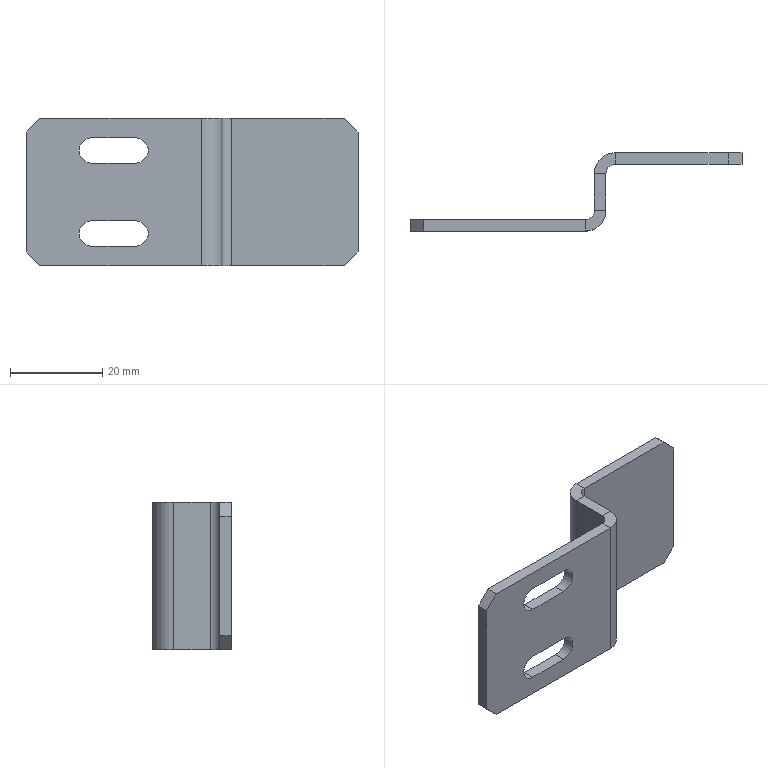Part | SolidWorks | features Chamfer 1, FlatPattern 1, HoleWzd 1, SMBaseFlange 1, SheetMetal 1 | 1 solid | 34 faces | box 72 x 17 x 32 mm | volume 6272 mm3 | plane 26 | cylinder 8 | commonest cylinder face diameters 5.5 x4 4 x2 9 x2
STEP:
#1=CARTESIAN_POINT('',(40.,2.,32.));
#2=VERTEX_POINT('',#1);
#3=CARTESIAN_POINT('',(42.5,2.,32.));
#4=VERTEX_POINT('',#3);
#5=CARTESIAN_POINT('',(40.,2.,32.));
#6=DIRECTION('',(1.,0.,0.));
#7=VECTOR('',#6,1000.);
#8=LINE('',#5,#7);
#9=EDGE_CURVE('',#2,#4,#8,.T.);
#10=ORIENTED_EDGE('',*,*,#9,.F.);
#11=CARTESIAN_POINT('',(38.,0.,32.));
#12=VERTEX_POINT('',#11);
#13=CARTESIAN_POINT('',(38.,2.,32.));
#14=DIRECTION('',(0.,0.,1.));
#15=DIRECTION('',(-1.,0.,0.));
#16=AXIS2_PLACEMENT_3D('',#13,#14,#15);
#17=CIRCLE('',#16,2.);
#18=EDGE_CURVE('',#12,#2,#17,.T.);
#19=ORIENTED_EDGE('',*,*,#18,.F.);
#20=CARTESIAN_POINT('',(38.,-2.5,32.));
#21=VERTEX_POINT('',#20);
#22=CARTESIAN_POINT('',(38.,-2.5,32.));
#23=DIRECTION('',(0.,1.,0.));
#24=VECTOR('',#23,1000.);
#25=LINE('',#22,#24);
#26=EDGE_CURVE('',#21,#12,#25,.T.);
#27=ORIENTED_EDGE('',*,*,#26,.F.);
#28=CARTESIAN_POINT('',(38.,2.,32.));
#29=DIRECTION('',(0.,0.,1.));
#30=DIRECTION('',(1.,0.,0.));
#31=AXIS2_PLACEMENT_3D('',#28,#29,#30);
#32=CIRCLE('',#31,4.5);
#33=EDGE_CURVE('',#21,#4,#32,.T.);
#34=ORIENTED_EDGE('',*,*,#33,.T.);
#35=EDGE_LOOP('',(#10,#19,#27,#34));
#36=FACE_OUTER_BOUND('',#35,.T.);
#37=CARTESIAN_POINT('',(40.,2.,32.));
#38=DIRECTION('',(0.,0.,1.));
#39=DIRECTION('',(1.,0.,0.));
#40=AXIS2_PLACEMENT_3D('',#37,#38,#39);
#41=PLANE('',#40);
#42=ADVANCED_FACE('',(#36),#41,.T.);
#43=CARTESIAN_POINT('',(40.,10.,32.));
#44=VERTEX_POINT('',#43);
#45=CARTESIAN_POINT('',(40.,0.,32.));
#46=DIRECTION('',(0.,1.,0.));
#47=VECTOR('',#46,1000.);
#48=LINE('',#45,#47);
#49=EDGE_CURVE('',#2,#44,#48,.T.);
#50=ORIENTED_EDGE('',*,*,#49,.F.);
#51=ORIENTED_EDGE('',*,*,#9,.T.);
#52=CARTESIAN_POINT('',(42.5,10.,32.));
#53=VERTEX_POINT('',#52);
#54=CARTESIAN_POINT('',(42.5,0.,32.));
#55=DIRECTION('',(0.,1.,0.));
#56=VECTOR('',#55,1000.);
#57=LINE('',#54,#56);
#58=EDGE_CURVE('',#4,#53,#57,.T.);
#59=ORIENTED_EDGE('',*,*,#58,.T.);
#60=CARTESIAN_POINT('',(42.5,10.,32.));
#61=DIRECTION('',(-1.,0.,0.));
#62=VECTOR('',#61,1000.);
#63=LINE('',#60,#62);
#64=EDGE_CURVE('',#53,#44,#63,.T.);
#65=ORIENTED_EDGE('',*,*,#64,.T.);
#66=EDGE_LOOP('',(#50,#51,#59,#65));
#67=FACE_OUTER_BOUND('',#66,.T.);
#68=CARTESIAN_POINT('',(38.,-2.5,32.));
#69=DIRECTION('',(0.,0.,1.));
#70=DIRECTION('',(1.,0.,0.));
#71=AXIS2_PLACEMENT_3D('',#68,#69,#70);
#72=PLANE('',#71);
#73=ADVANCED_FACE('',(#67),#72,.T.);
#74=CARTESIAN_POINT('',(38.,0.,0.));
#75=VERTEX_POINT('',#74);
#76=CARTESIAN_POINT('',(38.,-2.5,0.));
#77=VERTEX_POINT('',#76);
#78=CARTESIAN_POINT('',(38.,0.,0.));
#79=DIRECTION('',(0.,-1.,0.));
#80=VECTOR('',#79,1000.);
#81=LINE('',#78,#80);
#82=EDGE_CURVE('',#75,#77,#81,.T.);
#83=ORIENTED_EDGE('',*,*,#82,.F.);
#84=CARTESIAN_POINT('',(40.,2.,0.));
#85=VERTEX_POINT('',#84);
#86=CARTESIAN_POINT('',(38.,2.,0.));
#87=DIRECTION('',(0.,0.,1.));
#88=DIRECTION('',(-1.,0.,0.));
#89=AXIS2_PLACEMENT_3D('',#86,#87,#88);
#90=CIRCLE('',#89,2.);
#91=EDGE_CURVE('',#75,#85,#90,.T.);
#92=ORIENTED_EDGE('',*,*,#91,.T.);
#93=CARTESIAN_POINT('',(42.5,2.,0.));
#94=VERTEX_POINT('',#93);
#95=CARTESIAN_POINT('',(42.5,2.,0.));
#96=DIRECTION('',(-1.,0.,0.));
#97=VECTOR('',#96,1000.);
#98=LINE('',#95,#97);
#99=EDGE_CURVE('',#94,#85,#98,.T.);
#100=ORIENTED_EDGE('',*,*,#99,.F.);
#101=CARTESIAN_POINT('',(38.,2.,0.));
#102=DIRECTION('',(0.,0.,1.));
#103=DIRECTION('',(1.,0.,0.));
#104=AXIS2_PLACEMENT_3D('',#101,#102,#103);
#105=CIRCLE('',#104,4.5);
#106=EDGE_CURVE('',#77,#94,#105,.T.);
#107=ORIENTED_EDGE('',*,*,#106,.F.);
#108=EDGE_LOOP('',(#83,#92,#100,#107));
#109=FACE_OUTER_BOUND('',#108,.T.);
#110=CARTESIAN_POINT('',(38.,0.,0.));
#111=DIRECTION('',(0.,0.,-1.));
#112=DIRECTION('',(-1.,0.,0.));
#113=AXIS2_PLACEMENT_3D('',#110,#111,#112);
#114=PLANE('',#113);
#115=ADVANCED_FACE('',(#109),#114,.T.);
#116=CARTESIAN_POINT('',(3.,-2.5,0.));
#117=VERTEX_POINT('',#116);
#118=CARTESIAN_POINT('',(0.,-2.5,0.));
#119=DIRECTION('',(1.,0.,0.));
#120=VECTOR('',#119,1000.);
#121=LINE('',#118,#120);
#122=EDGE_CURVE('',#117,#77,#121,.T.);
#123=ORIENTED_EDGE('',*,*,#122,.F.);
#124=CARTESIAN_POINT('',(3.,0.,0.));
#125=VERTEX_POINT('',#124);
#126=CARTESIAN_POINT('',(3.,2.,0.));
#127=DIRECTION('',(0.,1.,0.));
#128=VECTOR('',#127,1000.);
#129=LINE('',#126,#128);
#130=EDGE_CURVE('',#117,#125,#129,.T.);
#131=ORIENTED_EDGE('',*,*,#130,.T.);
#132=CARTESIAN_POINT('',(0.,0.,0.));
#133=DIRECTION('',(1.,0.,0.));
#134=VECTOR('',#133,1000.);
#135=LINE('',#132,#134);
#136=EDGE_CURVE('',#125,#75,#135,.T.);
#137=ORIENTED_EDGE('',*,*,#136,.T.);
#138=ORIENTED_EDGE('',*,*,#82,.T.);
#139=EDGE_LOOP('',(#123,#131,#137,#138));
#140=FACE_OUTER_BOUND('',#139,.T.);
#141=CARTESIAN_POINT('',(42.5,2.,0.));
#142=DIRECTION('',(0.,0.,-1.));
#143=DIRECTION('',(-1.,0.,0.));
#144=AXIS2_PLACEMENT_3D('',#141,#142,#143);
#145=PLANE('',#144);
#146=ADVANCED_FACE('',(#140),#145,.T.);
#147=CARTESIAN_POINT('',(44.5,14.5,32.));
#148=VERTEX_POINT('',#147);
#149=CARTESIAN_POINT('',(44.5,12.,32.));
#150=VERTEX_POINT('',#149);
#151=CARTESIAN_POINT('',(44.5,14.5,32.));
#152=DIRECTION('',(0.,-1.,0.));
#153=VECTOR('',#152,1000.);
#154=LINE('',#151,#153);
#155=EDGE_CURVE('',#148,#150,#154,.T.);
#156=ORIENTED_EDGE('',*,*,#155,.F.);
#157=CARTESIAN_POINT('',(44.5,10.,32.));
#158=DIRECTION('',(0.,0.,-1.));
#159=DIRECTION('',(1.,0.,0.));
#160=AXIS2_PLACEMENT_3D('',#157,#158,#159);
#161=CIRCLE('',#160,4.5);
#162=EDGE_CURVE('',#44,#148,#161,.T.);
#163=ORIENTED_EDGE('',*,*,#162,.F.);
#164=ORIENTED_EDGE('',*,*,#64,.F.);
#165=CARTESIAN_POINT('',(44.5,10.,32.));
#166=DIRECTION('',(0.,0.,-1.));
#167=DIRECTION('',(1.,0.,0.));
#168=AXIS2_PLACEMENT_3D('',#165,#166,#167);
#169=CIRCLE('',#168,2.);
#170=EDGE_CURVE('',#53,#150,#169,.T.);
#171=ORIENTED_EDGE('',*,*,#170,.T.);
#172=EDGE_LOOP('',(#156,#163,#164,#171));
#173=FACE_OUTER_BOUND('',#172,.T.);
#174=CARTESIAN_POINT('',(44.5,14.5,32.));
#175=DIRECTION('',(0.,0.,1.));
#176=DIRECTION('',(1.,0.,0.));
#177=AXIS2_PLACEMENT_3D('',#174,#175,#176);
#178=PLANE('',#177);
#179=ADVANCED_FACE('',(#173),#178,.T.);
#180=CARTESIAN_POINT('',(69.,12.,32.));
#181=VERTEX_POINT('',#180);
#182=CARTESIAN_POINT('',(40.,12.,32.));
#183=DIRECTION('',(1.,0.,0.));
#184=VECTOR('',#183,1000.);
#185=LINE('',#182,#184);
#186=EDGE_CURVE('',#150,#181,#185,.T.);
#187=ORIENTED_EDGE('',*,*,#186,.T.);
#188=CARTESIAN_POINT('',(69.,14.5,32.));
#189=VERTEX_POINT('',#188);
#190=CARTESIAN_POINT('',(69.,10.,32.));
#191=DIRECTION('',(0.,1.,0.));
#192=VECTOR('',#191,1000.);
#193=LINE('',#190,#192);
#194=EDGE_CURVE('',#181,#189,#193,.T.);
#195=ORIENTED_EDGE('',*,*,#194,.T.);
#196=CARTESIAN_POINT('',(40.,14.5,32.));
#197=DIRECTION('',(1.,0.,0.));
#198=VECTOR('',#197,1000.);
#199=LINE('',#196,#198);
#200=EDGE_CURVE('',#148,#189,#199,.T.);
#201=ORIENTED_EDGE('',*,*,#200,.F.);
#202=ORIENTED_EDGE('',*,*,#155,.T.);
#203=EDGE_LOOP('',(#187,#195,#201,#202));
#204=FACE_OUTER_BOUND('',#203,.T.);
#205=CARTESIAN_POINT('',(42.5,10.,32.));
#206=DIRECTION('',(0.,0.,1.));
#207=DIRECTION('',(1.,0.,0.));
#208=AXIS2_PLACEMENT_3D('',#205,#206,#207);
#209=PLANE('',#208);
#210=ADVANCED_FACE('',(#204),#209,.T.);
#211=CARTESIAN_POINT('',(40.,10.,0.));
#212=VERTEX_POINT('',#211);
#213=CARTESIAN_POINT('',(42.5,10.,0.));
#214=VERTEX_POINT('',#213);
#215=CARTESIAN_POINT('',(40.,10.,0.));
#216=DIRECTION('',(1.,0.,0.));
#217=VECTOR('',#216,1000.);
#218=LINE('',#215,#217);
#219=EDGE_CURVE('',#212,#214,#218,.T.);
#220=ORIENTED_EDGE('',*,*,#219,.F.);
#221=CARTESIAN_POINT('',(44.5,14.5,0.));
#222=VERTEX_POINT('',#221);
#223=CARTESIAN_POINT('',(44.5,10.,0.));
#224=DIRECTION('',(0.,0.,-1.));
#225=DIRECTION('',(1.,0.,0.));
#226=AXIS2_PLACEMENT_3D('',#223,#224,#225);
#227=CIRCLE('',#226,4.5);
#228=EDGE_CURVE('',#212,#222,#227,.T.);
#229=ORIENTED_EDGE('',*,*,#228,.T.);
#230=CARTESIAN_POINT('',(44.5,12.,0.));
#231=VERTEX_POINT('',#230);
#232=CARTESIAN_POINT('',(44.5,12.,0.));
#233=DIRECTION('',(0.,1.,0.));
#234=VECTOR('',#233,1000.);
#235=LINE('',#232,#234);
#236=EDGE_CURVE('',#231,#222,#235,.T.);
#237=ORIENTED_EDGE('',*,*,#236,.F.);
#238=CARTESIAN_POINT('',(44.5,10.,0.));
#239=DIRECTION('',(0.,0.,-1.));
#240=DIRECTION('',(1.,0.,0.));
#241=AXIS2_PLACEMENT_3D('',#238,#239,#240);
#242=CIRCLE('',#241,2.);
#243=EDGE_CURVE('',#214,#231,#242,.T.);
#244=ORIENTED_EDGE('',*,*,#243,.F.);
#245=EDGE_LOOP('',(#220,#229,#237,#244));
#246=FACE_OUTER_BOUND('',#245,.T.);
#247=CARTESIAN_POINT('',(40.,10.,0.));
#248=DIRECTION('',(0.,0.,-1.));
#249=DIRECTION('',(-1.,0.,0.));
#250=AXIS2_PLACEMENT_3D('',#247,#248,#249);
#251=PLANE('',#250);
#252=ADVANCED_FACE('',(#246),#251,.T.);
#253=CARTESIAN_POINT('',(40.,0.,0.));
#254=DIRECTION('',(0.,1.,0.));
#255=VECTOR('',#254,1000.);
#256=LINE('',#253,#255);
#257=EDGE_CURVE('',#85,#212,#256,.T.);
#258=ORIENTED_EDGE('',*,*,#257,.T.);
#259=ORIENTED_EDGE('',*,*,#219,.T.);
#260=CARTESIAN_POINT('',(42.5,0.,0.));
#261=DIRECTION('',(0.,1.,0.));
#262=VECTOR('',#261,1000.);
#263=LINE('',#260,#262);
#264=EDGE_CURVE('',#94,#214,#263,.T.);
#265=ORIENTED_EDGE('',*,*,#264,.F.);
#266=ORIENTED_EDGE('',*,*,#99,.T.);
#267=EDGE_LOOP('',(#258,#259,#265,#266));
#268=FACE_OUTER_BOUND('',#267,.T.);
#269=CARTESIAN_POINT('',(44.5,12.,0.));
#270=DIRECTION('',(0.,0.,-1.));
#271=DIRECTION('',(-1.,0.,0.));
#272=AXIS2_PLACEMENT_3D('',#269,#270,#271);
#273=PLANE('',#272);
#274=ADVANCED_FACE('',(#268),#273,.T.);
#275=CARTESIAN_POINT('',(72.,12.,29.));
#276=VERTEX_POINT('',#275);
#277=CARTESIAN_POINT('',(72.,12.,3.));
#278=VERTEX_POINT('',#277);
#279=CARTESIAN_POINT('',(72.,12.,32.));
#280=DIRECTION('',(0.,0.,-1.));
#281=VECTOR('',#280,1000.);
#282=LINE('',#279,#281);
#283=EDGE_CURVE('',#276,#278,#282,.T.);
#284=ORIENTED_EDGE('',*,*,#283,.F.);
#285=CARTESIAN_POINT('',(72.,12.,29.));
#286=DIRECTION('',(-0.7071,0.,0.7071));
#287=VECTOR('',#286,1000.);
#288=LINE('',#285,#287);
#289=EDGE_CURVE('',#276,#181,#288,.T.);
#290=ORIENTED_EDGE('',*,*,#289,.T.);
#291=ORIENTED_EDGE('',*,*,#186,.F.);
#292=CARTESIAN_POINT('',(44.5,12.,32.));
#293=DIRECTION('',(0.,0.,-1.));
#294=VECTOR('',#293,1000.);
#295=LINE('',#292,#294);
#296=EDGE_CURVE('',#150,#231,#295,.T.);
#297=ORIENTED_EDGE('',*,*,#296,.T.);
#298=CARTESIAN_POINT('',(69.,12.,0.));
#299=VERTEX_POINT('',#298);
#300=CARTESIAN_POINT('',(40.,12.,0.));
#301=DIRECTION('',(1.,0.,0.));
#302=VECTOR('',#301,1000.);
#303=LINE('',#300,#302);
#304=EDGE_CURVE('',#231,#299,#303,.T.);
#305=ORIENTED_EDGE('',*,*,#304,.T.);
#306=CARTESIAN_POINT('',(69.,12.,0.));
#307=DIRECTION('',(0.7071,0.,0.7071));
#308=VECTOR('',#307,1000.);
#309=LINE('',#306,#308);
#310=EDGE_CURVE('',#299,#278,#309,.T.);
#311=ORIENTED_EDGE('',*,*,#310,.T.);
#312=EDGE_LOOP('',(#284,#290,#291,#297,#305,#311));
#313=FACE_OUTER_BOUND('',#312,.T.);
#314=CARTESIAN_POINT('',(40.,12.,32.));
#315=DIRECTION('',(0.,1.,0.));
#316=DIRECTION('',(0.,0.,1.));
#317=AXIS2_PLACEMENT_3D('',#314,#315,#316);
#318=PLANE('',#317);
#319=ADVANCED_FACE('',(#313),#318,.F.);
#320=CARTESIAN_POINT('',(72.,14.5,29.));
#321=VERTEX_POINT('',#320);
#322=CARTESIAN_POINT('',(72.,14.5,3.));
#323=VERTEX_POINT('',#322);
#324=CARTESIAN_POINT('',(72.,14.5,32.));
#325=DIRECTION('',(0.,0.,-1.));
#326=VECTOR('',#325,1000.);
#327=LINE('',#324,#326);
#328=EDGE_CURVE('',#321,#323,#327,.T.);
#329=ORIENTED_EDGE('',*,*,#328,.F.);
#330=CARTESIAN_POINT('',(72.,14.5,29.));
#331=DIRECTION('',(0.,-1.,0.));
#332=VECTOR('',#331,1000.);
#333=LINE('',#330,#332);
#334=EDGE_CURVE('',#321,#276,#333,.T.);
#335=ORIENTED_EDGE('',*,*,#334,.T.);
#336=ORIENTED_EDGE('',*,*,#283,.T.);
#337=CARTESIAN_POINT('',(72.,14.5,3.));
#338=DIRECTION('',(0.,1.,0.));
#339=VECTOR('',#338,1000.);
#340=LINE('',#337,#339);
#341=EDGE_CURVE('',#278,#323,#340,.T.);
#342=ORIENTED_EDGE('',*,*,#341,.T.);
#343=EDGE_LOOP('',(#329,#335,#336,#342));
#344=FACE_OUTER_BOUND('',#343,.T.);
#345=CARTESIAN_POINT('',(72.,14.5,32.));
#346=DIRECTION('',(1.,0.,0.));
#347=DIRECTION('',(0.,0.,-1.));
#348=AXIS2_PLACEMENT_3D('',#345,#346,#347);
#349=PLANE('',#348);
#350=ADVANCED_FACE('',(#344),#349,.T.);
#351=ORIENTED_EDGE('',*,*,#200,.T.);
#352=CARTESIAN_POINT('',(54.5,14.5,46.5));
#353=DIRECTION('',(0.7071,0.,-0.7071));
#354=VECTOR('',#353,1000.);
#355=LINE('',#352,#354);
#356=EDGE_CURVE('',#189,#321,#355,.T.);
#357=ORIENTED_EDGE('',*,*,#356,.T.);
#358=ORIENTED_EDGE('',*,*,#328,.T.);
#359=CARTESIAN_POINT('',(69.,14.5,0.));
#360=VERTEX_POINT('',#359);
#361=CARTESIAN_POINT('',(70.5,14.5,1.5));
#362=DIRECTION('',(-0.7071,0.,-0.7071));
#363=VECTOR('',#362,1000.);
#364=LINE('',#361,#363);
#365=EDGE_CURVE('',#323,#360,#364,.T.);
#366=ORIENTED_EDGE('',*,*,#365,.T.);
#367=CARTESIAN_POINT('',(40.,14.5,0.));
#368=DIRECTION('',(1.,0.,0.));
#369=VECTOR('',#368,1000.);
#370=LINE('',#367,#369);
#371=EDGE_CURVE('',#222,#360,#370,.T.);
#372=ORIENTED_EDGE('',*,*,#371,.F.);
#373=CARTESIAN_POINT('',(44.5,14.5,32.));
#374=DIRECTION('',(0.,0.,-1.));
#375=VECTOR('',#374,1000.);
#376=LINE('',#373,#375);
#377=EDGE_CURVE('',#148,#222,#376,.T.);
#378=ORIENTED_EDGE('',*,*,#377,.F.);
#379=EDGE_LOOP('',(#351,#357,#358,#366,#372,#378));
#380=FACE_OUTER_BOUND('',#379,.T.);
#381=CARTESIAN_POINT('',(40.,14.5,32.));
#382=DIRECTION('',(0.,1.,0.));
#383=DIRECTION('',(0.,0.,1.));
#384=AXIS2_PLACEMENT_3D('',#381,#382,#383);
#385=PLANE('',#384);
#386=ADVANCED_FACE('',(#380),#385,.T.);
#387=ORIENTED_EDGE('',*,*,#228,.F.);
#388=CARTESIAN_POINT('',(40.,10.,32.));
#389=DIRECTION('',(0.,0.,-1.));
#390=VECTOR('',#389,1000.);
#391=LINE('',#388,#390);
#392=EDGE_CURVE('',#44,#212,#391,.T.);
#393=ORIENTED_EDGE('',*,*,#392,.F.);
#394=ORIENTED_EDGE('',*,*,#162,.T.);
#395=ORIENTED_EDGE('',*,*,#377,.T.);
#396=EDGE_LOOP('',(#387,#393,#394,#395));
#397=FACE_OUTER_BOUND('',#396,.T.);
#398=CARTESIAN_POINT('',(44.5,10.,32.));
#399=DIRECTION('',(0.,0.,-1.));
#400=DIRECTION('',(-1.,0.,0.));
#401=AXIS2_PLACEMENT_3D('',#398,#399,#400);
#402=CYLINDRICAL_SURFACE('',#401,4.5);
#403=ADVANCED_FACE('',(#397),#402,.T.);
#404=ORIENTED_EDGE('',*,*,#257,.F.);
#405=CARTESIAN_POINT('',(40.,2.,32.));
#406=DIRECTION('',(0.,0.,-1.));
#407=VECTOR('',#406,1000.);
#408=LINE('',#405,#407);
#409=EDGE_CURVE('',#2,#85,#408,.T.);
#410=ORIENTED_EDGE('',*,*,#409,.F.);
#411=ORIENTED_EDGE('',*,*,#49,.T.);
#412=ORIENTED_EDGE('',*,*,#392,.T.);
#413=EDGE_LOOP('',(#404,#410,#411,#412));
#414=FACE_OUTER_BOUND('',#413,.T.);
#415=CARTESIAN_POINT('',(40.,0.,32.));
#416=DIRECTION('',(-1.,0.,0.));
#417=DIRECTION('',(0.,0.,1.));
#418=AXIS2_PLACEMENT_3D('',#415,#416,#417);
#419=PLANE('',#418);
#420=ADVANCED_FACE('',(#414),#419,.T.);
#421=ORIENTED_EDGE('',*,*,#91,.F.);
#422=CARTESIAN_POINT('',(38.,0.,32.));
#423=DIRECTION('',(0.,0.,-1.));
#424=VECTOR('',#423,1000.);
#425=LINE('',#422,#424);
#426=EDGE_CURVE('',#12,#75,#425,.T.);
#427=ORIENTED_EDGE('',*,*,#426,.F.);
#428=ORIENTED_EDGE('',*,*,#18,.T.);
#429=ORIENTED_EDGE('',*,*,#409,.T.);
#430=EDGE_LOOP('',(#421,#427,#428,#429));
#431=FACE_OUTER_BOUND('',#430,.T.);
#432=CARTESIAN_POINT('',(38.,2.,32.));
#433=DIRECTION('',(0.,0.,-1.));
#434=DIRECTION('',(-1.,0.,0.));
#435=AXIS2_PLACEMENT_3D('',#432,#433,#434);
#436=CYLINDRICAL_SURFACE('',#435,2.);
#437=ADVANCED_FACE('',(#431),#436,.F.);
#438=CARTESIAN_POINT('',(14.25,0.,9.75));
#439=VERTEX_POINT('',#438);
#440=CARTESIAN_POINT('',(23.75,0.,9.75));
#441=VERTEX_POINT('',#440);
#442=CARTESIAN_POINT('',(14.25,0.,9.75));
#443=DIRECTION('',(1.,0.,0.));
#444=VECTOR('',#443,1000.);
#445=LINE('',#442,#444);
#446=EDGE_CURVE('',#439,#441,#445,.T.);
#447=ORIENTED_EDGE('',*,*,#446,.F.);
#448=CARTESIAN_POINT('',(14.25,0.,4.25));
#449=VERTEX_POINT('',#448);
#450=CARTESIAN_POINT('',(14.25,0.,7.));
#451=DIRECTION('',(0.,1.,0.));
#452=DIRECTION('',(0.,0.,1.));
#453=AXIS2_PLACEMENT_3D('',#450,#451,#452);
#454=CIRCLE('',#453,2.75);
#455=EDGE_CURVE('',#449,#439,#454,.T.);
#456=ORIENTED_EDGE('',*,*,#455,.F.);
#457=CARTESIAN_POINT('',(23.75,0.,4.25));
#458=VERTEX_POINT('',#457);
#459=CARTESIAN_POINT('',(14.25,0.,4.25));
#460=DIRECTION('',(1.,0.,0.));
#461=VECTOR('',#460,1000.);
#462=LINE('',#459,#461);
#463=EDGE_CURVE('',#449,#458,#462,.T.);
#464=ORIENTED_EDGE('',*,*,#463,.T.);
#465=CARTESIAN_POINT('',(23.75,0.,7.));
#466=DIRECTION('',(0.,1.,0.));
#467=DIRECTION('',(0.,0.,1.));
#468=AXIS2_PLACEMENT_3D('',#465,#466,#467);
#469=CIRCLE('',#468,2.75);
#470=EDGE_CURVE('',#441,#458,#469,.T.);
#471=ORIENTED_EDGE('',*,*,#470,.F.);
#472=EDGE_LOOP('',(#447,#456,#464,#471));
#473=FACE_BOUND('',#472,.T.);
#474=CARTESIAN_POINT('',(23.75,0.,27.75));
#475=VERTEX_POINT('',#474);
#476=CARTESIAN_POINT('',(23.75,0.,22.25));
#477=VERTEX_POINT('',#476);
#478=CARTESIAN_POINT('',(23.75,0.,25.));
#479=DIRECTION('',(0.,1.,0.));
#480=DIRECTION('',(0.,0.,1.));
#481=AXIS2_PLACEMENT_3D('',#478,#479,#480);
#482=CIRCLE('',#481,2.75);
#483=EDGE_CURVE('',#475,#477,#482,.T.);
#484=ORIENTED_EDGE('',*,*,#483,.F.);
#485=CARTESIAN_POINT('',(14.25,0.,27.75));
#486=VERTEX_POINT('',#485);
#487=CARTESIAN_POINT('',(14.25,0.,27.75));
#488=DIRECTION('',(1.,0.,0.));
#489=VECTOR('',#488,1000.);
#490=LINE('',#487,#489);
#491=EDGE_CURVE('',#486,#475,#490,.T.);
#492=ORIENTED_EDGE('',*,*,#491,.F.);
#493=CARTESIAN_POINT('',(14.25,0.,22.25));
#494=VERTEX_POINT('',#493);
#495=CARTESIAN_POINT('',(14.25,0.,25.));
#496=DIRECTION('',(0.,1.,0.));
#497=DIRECTION('',(0.,0.,1.));
#498=AXIS2_PLACEMENT_3D('',#495,#496,#497);
#499=CIRCLE('',#498,2.75);
#500=EDGE_CURVE('',#494,#486,#499,.T.);
#501=ORIENTED_EDGE('',*,*,#500,.F.);
#502=CARTESIAN_POINT('',(14.25,0.,22.25));
#503=DIRECTION('',(1.,0.,0.));
#504=VECTOR('',#503,1000.);
#505=LINE('',#502,#504);
#506=EDGE_CURVE('',#494,#477,#505,.T.);
#507=ORIENTED_EDGE('',*,*,#506,.T.);
#508=EDGE_LOOP('',(#484,#492,#501,#507));
#509=FACE_BOUND('',#508,.T.);
#510=CARTESIAN_POINT('',(0.,0.,29.));
#511=VERTEX_POINT('',#510);
#512=CARTESIAN_POINT('',(0.,0.,3.));
#513=VERTEX_POINT('',#512);
#514=CARTESIAN_POINT('',(0.,0.,32.));
#515=DIRECTION('',(0.,0.,-1.));
#516=VECTOR('',#515,1000.);
#517=LINE('',#514,#516);
#518=EDGE_CURVE('',#511,#513,#517,.T.);
#519=ORIENTED_EDGE('',*,*,#518,.F.);
#520=CARTESIAN_POINT('',(3.,0.,32.));
#521=VERTEX_POINT('',#520);
#522=CARTESIAN_POINT('',(1.5,0.,30.5));
#523=DIRECTION('',(0.7071,0.,0.7071));
#524=VECTOR('',#523,1000.);
#525=LINE('',#522,#524);
#526=EDGE_CURVE('',#511,#521,#525,.T.);
#527=ORIENTED_EDGE('',*,*,#526,.T.);
#528=CARTESIAN_POINT('',(0.,0.,32.));
#529=DIRECTION('',(1.,0.,0.));
#530=VECTOR('',#529,1000.);
#531=LINE('',#528,#530);
#532=EDGE_CURVE('',#521,#12,#531,.T.);
#533=ORIENTED_EDGE('',*,*,#532,.T.);
#534=ORIENTED_EDGE('',*,*,#426,.T.);
#535=ORIENTED_EDGE('',*,*,#136,.F.);
#536=CARTESIAN_POINT('',(-14.5,0.,17.5));
#537=DIRECTION('',(-0.7071,0.,0.7071));
#538=VECTOR('',#537,1000.);
#539=LINE('',#536,#538);
#540=EDGE_CURVE('',#125,#513,#539,.T.);
#541=ORIENTED_EDGE('',*,*,#540,.T.);
#542=EDGE_LOOP('',(#519,#527,#533,#534,#535,#541));
#543=FACE_OUTER_BOUND('',#542,.T.);
#544=CARTESIAN_POINT('',(0.,0.,32.));
#545=DIRECTION('',(0.,1.,0.));
#546=DIRECTION('',(0.,0.,1.));
#547=AXIS2_PLACEMENT_3D('',#544,#545,#546);
#548=PLANE('',#547);
#549=ADVANCED_FACE('',(#473,#509,#543),#548,.T.);
#550=CARTESIAN_POINT('',(0.,-2.5,29.));
#551=VERTEX_POINT('',#550);
#552=CARTESIAN_POINT('',(0.,-2.5,3.));
#553=VERTEX_POINT('',#552);
#554=CARTESIAN_POINT('',(0.,-2.5,32.));
#555=DIRECTION('',(0.,0.,-1.));
#556=VECTOR('',#555,1000.);
#557=LINE('',#554,#556);
#558=EDGE_CURVE('',#551,#553,#557,.T.);
#559=ORIENTED_EDGE('',*,*,#558,.F.);
#560=CARTESIAN_POINT('',(0.,-2.5,29.));
#561=DIRECTION('',(0.,1.,0.));
#562=VECTOR('',#561,1000.);
#563=LINE('',#560,#562);
#564=EDGE_CURVE('',#551,#511,#563,.T.);
#565=ORIENTED_EDGE('',*,*,#564,.T.);
#566=ORIENTED_EDGE('',*,*,#518,.T.);
#567=CARTESIAN_POINT('',(0.,-2.5,3.));
#568=DIRECTION('',(0.,-1.,0.));
#569=VECTOR('',#568,1000.);
#570=LINE('',#567,#569);
#571=EDGE_CURVE('',#513,#553,#570,.T.);
#572=ORIENTED_EDGE('',*,*,#571,.T.);
#573=EDGE_LOOP('',(#559,#565,#566,#572));
#574=FACE_OUTER_BOUND('',#573,.T.);
#575=CARTESIAN_POINT('',(0.,-2.5,32.));
#576=DIRECTION('',(-1.,0.,0.));
#577=DIRECTION('',(0.,0.,1.));
#578=AXIS2_PLACEMENT_3D('',#575,#576,#577);
#579=PLANE('',#578);
#580=ADVANCED_FACE('',(#574),#579,.T.);
#581=CARTESIAN_POINT('',(14.25,-2.5,9.75));
#582=VERTEX_POINT('',#581);
#583=CARTESIAN_POINT('',(23.75,-2.5,9.75));
#584=VERTEX_POINT('',#583);
#585=CARTESIAN_POINT('',(14.25,-2.5,9.75));
#586=DIRECTION('',(1.,0.,0.));
#587=VECTOR('',#586,1000.);
#588=LINE('',#585,#587);
#589=EDGE_CURVE('',#582,#584,#588,.T.);
#590=ORIENTED_EDGE('',*,*,#589,.T.);
#591=CARTESIAN_POINT('',(23.75,-2.5,4.25));
#592=VERTEX_POINT('',#591);
#593=CARTESIAN_POINT('',(23.75,-2.5,7.));
#594=DIRECTION('',(0.,1.,0.));
#595=DIRECTION('',(0.,0.,1.));
#596=AXIS2_PLACEMENT_3D('',#593,#594,#595);
#597=CIRCLE('',#596,2.75);
#598=EDGE_CURVE('',#584,#592,#597,.T.);
#599=ORIENTED_EDGE('',*,*,#598,.T.);
#600=CARTESIAN_POINT('',(14.25,-2.5,4.25));
#601=VERTEX_POINT('',#600);
#602=CARTESIAN_POINT('',(14.25,-2.5,4.25));
#603=DIRECTION('',(1.,0.,0.));
#604=VECTOR('',#603,1000.);
#605=LINE('',#602,#604);
#606=EDGE_CURVE('',#601,#592,#605,.T.);
#607=ORIENTED_EDGE('',*,*,#606,.F.);
#608=CARTESIAN_POINT('',(14.25,-2.5,7.));
#609=DIRECTION('',(0.,1.,0.));
#610=DIRECTION('',(0.,0.,1.));
#611=AXIS2_PLACEMENT_3D('',#608,#609,#610);
#612=CIRCLE('',#611,2.75);
#613=EDGE_CURVE('',#601,#582,#612,.T.);
#614=ORIENTED_EDGE('',*,*,#613,.T.);
#615=EDGE_LOOP('',(#590,#599,#607,#614));
#616=FACE_BOUND('',#615,.T.);
#617=CARTESIAN_POINT('',(14.25,-2.5,27.75));
#618=VERTEX_POINT('',#617);
#619=CARTESIAN_POINT('',(23.75,-2.5,27.75));
#620=VERTEX_POINT('',#619);
#621=CARTESIAN_POINT('',(14.25,-2.5,27.75));
#622=DIRECTION('',(1.,0.,0.));
#623=VECTOR('',#622,1000.);
#624=LINE('',#621,#623);
#625=EDGE_CURVE('',#618,#620,#624,.T.);
#626=ORIENTED_EDGE('',*,*,#625,.T.);
#627=CARTESIAN_POINT('',(23.75,-2.5,22.25));
#628=VERTEX_POINT('',#627);
#629=CARTESIAN_POINT('',(23.75,-2.5,25.));
#630=DIRECTION('',(0.,1.,0.));
#631=DIRECTION('',(0.,0.,1.));
#632=AXIS2_PLACEMENT_3D('',#629,#630,#631);
#633=CIRCLE('',#632,2.75);
#634=EDGE_CURVE('',#620,#628,#633,.T.);
#635=ORIENTED_EDGE('',*,*,#634,.T.);
#636=CARTESIAN_POINT('',(14.25,-2.5,22.25));
#637=VERTEX_POINT('',#636);
#638=CARTESIAN_POINT('',(14.25,-2.5,22.25));
#639=DIRECTION('',(1.,0.,0.));
#640=VECTOR('',#639,1000.);
#641=LINE('',#638,#640);
#642=EDGE_CURVE('',#637,#628,#641,.T.);
#643=ORIENTED_EDGE('',*,*,#642,.F.);
#644=CARTESIAN_POINT('',(14.25,-2.5,25.));
#645=DIRECTION('',(0.,1.,0.));
#646=DIRECTION('',(0.,0.,1.));
#647=AXIS2_PLACEMENT_3D('',#644,#645,#646);
#648=CIRCLE('',#647,2.75);
#649=EDGE_CURVE('',#637,#618,#648,.T.);
#650=ORIENTED_EDGE('',*,*,#649,.T.);
#651=EDGE_LOOP('',(#626,#635,#643,#650));
#652=FACE_BOUND('',#651,.T.);
#653=CARTESIAN_POINT('',(3.,-2.5,32.));
#654=VERTEX_POINT('',#653);
#655=CARTESIAN_POINT('',(0.,-2.5,32.));
#656=DIRECTION('',(1.,0.,0.));
#657=VECTOR('',#656,1000.);
#658=LINE('',#655,#657);
#659=EDGE_CURVE('',#654,#21,#658,.T.);
#660=ORIENTED_EDGE('',*,*,#659,.F.);
#661=CARTESIAN_POINT('',(0.,-2.5,29.));
#662=DIRECTION('',(-0.7071,0.,-0.7071));
#663=VECTOR('',#662,1000.);
#664=LINE('',#661,#663);
#665=EDGE_CURVE('',#654,#551,#664,.T.);
#666=ORIENTED_EDGE('',*,*,#665,.T.);
#667=ORIENTED_EDGE('',*,*,#558,.T.);
#668=CARTESIAN_POINT('',(3.,-2.5,0.));
#669=DIRECTION('',(0.7071,0.,-0.7071));
#670=VECTOR('',#669,1000.);
#671=LINE('',#668,#670);
#672=EDGE_CURVE('',#553,#117,#671,.T.);
#673=ORIENTED_EDGE('',*,*,#672,.T.);
#674=ORIENTED_EDGE('',*,*,#122,.T.);
#675=CARTESIAN_POINT('',(38.,-2.5,32.));
#676=DIRECTION('',(0.,0.,-1.));
#677=VECTOR('',#676,1000.);
#678=LINE('',#675,#677);
#679=EDGE_CURVE('',#21,#77,#678,.T.);
#680=ORIENTED_EDGE('',*,*,#679,.F.);
#681=EDGE_LOOP('',(#660,#666,#667,#673,#674,#680));
#682=FACE_OUTER_BOUND('',#681,.T.);
#683=CARTESIAN_POINT('',(0.,-2.5,32.));
#684=DIRECTION('',(0.,1.,0.));
#685=DIRECTION('',(0.,0.,1.));
#686=AXIS2_PLACEMENT_3D('',#683,#684,#685);
#687=PLANE('',#686);
#688=ADVANCED_FACE('',(#616,#652,#682),#687,.F.);
#689=ORIENTED_EDGE('',*,*,#106,.T.);
#690=CARTESIAN_POINT('',(42.5,2.,32.));
#691=DIRECTION('',(0.,0.,-1.));
#692=VECTOR('',#691,1000.);
#693=LINE('',#690,#692);
#694=EDGE_CURVE('',#4,#94,#693,.T.);
#695=ORIENTED_EDGE('',*,*,#694,.F.);
#696=ORIENTED_EDGE('',*,*,#33,.F.);
#697=ORIENTED_EDGE('',*,*,#679,.T.);
#698=EDGE_LOOP('',(#689,#695,#696,#697));
#699=FACE_OUTER_BOUND('',#698,.T.);
#700=CARTESIAN_POINT('',(38.,2.,32.));
#701=DIRECTION('',(0.,0.,-1.));
#702=DIRECTION('',(-1.,0.,0.));
#703=AXIS2_PLACEMENT_3D('',#700,#701,#702);
#704=CYLINDRICAL_SURFACE('',#703,4.5);
#705=ADVANCED_FACE('',(#699),#704,.T.);
#706=ORIENTED_EDGE('',*,*,#264,.T.);
#707=CARTESIAN_POINT('',(42.5,10.,32.));
#708=DIRECTION('',(0.,0.,-1.));
#709=VECTOR('',#708,1000.);
#710=LINE('',#707,#709);
#711=EDGE_CURVE('',#53,#214,#710,.T.);
#712=ORIENTED_EDGE('',*,*,#711,.F.);
#713=ORIENTED_EDGE('',*,*,#58,.F.);
#714=ORIENTED_EDGE('',*,*,#694,.T.);
#715=EDGE_LOOP('',(#706,#712,#713,#714));
#716=FACE_OUTER_BOUND('',#715,.T.);
#717=CARTESIAN_POINT('',(42.5,0.,32.));
#718=DIRECTION('',(-1.,0.,0.));
#719=DIRECTION('',(0.,0.,1.));
#720=AXIS2_PLACEMENT_3D('',#717,#718,#719);
#721=PLANE('',#720);
#722=ADVANCED_FACE('',(#716),#721,.F.);
#723=ORIENTED_EDGE('',*,*,#243,.T.);
#724=ORIENTED_EDGE('',*,*,#296,.F.);
#725=ORIENTED_EDGE('',*,*,#170,.F.);
#726=ORIENTED_EDGE('',*,*,#711,.T.);
#727=EDGE_LOOP('',(#723,#724,#725,#726));
#728=FACE_OUTER_BOUND('',#727,.T.);
#729=CARTESIAN_POINT('',(44.5,10.,32.));
#730=DIRECTION('',(0.,0.,-1.));
#731=DIRECTION('',(-1.,0.,0.));
#732=AXIS2_PLACEMENT_3D('',#729,#730,#731);
#733=CYLINDRICAL_SURFACE('',#732,2.);
#734=ADVANCED_FACE('',(#728),#733,.F.);
#735=ORIENTED_EDGE('',*,*,#532,.F.);
#736=CARTESIAN_POINT('',(3.,10.,32.));
#737=DIRECTION('',(0.,-1.,0.));
#738=VECTOR('',#737,1000.);
#739=LINE('',#736,#738);
#740=EDGE_CURVE('',#521,#654,#739,.T.);
#741=ORIENTED_EDGE('',*,*,#740,.T.);
#742=ORIENTED_EDGE('',*,*,#659,.T.);
#743=ORIENTED_EDGE('',*,*,#26,.T.);
#744=EDGE_LOOP('',(#735,#741,#742,#743));
#745=FACE_OUTER_BOUND('',#744,.T.);
#746=CARTESIAN_POINT('',(44.5,10.,32.));
#747=DIRECTION('',(0.,0.,1.));
#748=DIRECTION('',(1.,0.,0.));
#749=AXIS2_PLACEMENT_3D('',#746,#747,#748);
#750=PLANE('',#749);
#751=ADVANCED_FACE('',(#745),#750,.T.);
#752=ORIENTED_EDGE('',*,*,#371,.T.);
#753=CARTESIAN_POINT('',(69.,12.,0.));
#754=DIRECTION('',(0.,-1.,0.));
#755=VECTOR('',#754,1000.);
#756=LINE('',#753,#755);
#757=EDGE_CURVE('',#360,#299,#756,.T.);
#758=ORIENTED_EDGE('',*,*,#757,.T.);
#759=ORIENTED_EDGE('',*,*,#304,.F.);
#760=ORIENTED_EDGE('',*,*,#236,.T.);
#761=EDGE_LOOP('',(#752,#758,#759,#760));
#762=FACE_OUTER_BOUND('',#761,.T.);
#763=CARTESIAN_POINT('',(44.5,10.,0.));
#764=DIRECTION('',(0.,0.,1.));
#765=DIRECTION('',(1.,0.,0.));
#766=AXIS2_PLACEMENT_3D('',#763,#764,#765);
#767=PLANE('',#766);
#768=ADVANCED_FACE('',(#762),#767,.F.);
#769=ORIENTED_EDGE('',*,*,#634,.F.);
#770=CARTESIAN_POINT('',(23.75,0.,27.75));
#771=DIRECTION('',(0.,-1.,0.));
#772=VECTOR('',#771,1000.);
#773=LINE('',#770,#772);
#774=EDGE_CURVE('',#475,#620,#773,.T.);
#775=ORIENTED_EDGE('',*,*,#774,.F.);
#776=ORIENTED_EDGE('',*,*,#483,.T.);
#777=CARTESIAN_POINT('',(23.75,0.,22.25));
#778=DIRECTION('',(0.,1.,0.));
#779=VECTOR('',#778,1000.);
#780=LINE('',#777,#779);
#781=EDGE_CURVE('',#628,#477,#780,.T.);
#782=ORIENTED_EDGE('',*,*,#781,.F.);
#783=EDGE_LOOP('',(#769,#775,#776,#782));
#784=FACE_OUTER_BOUND('',#783,.T.);
#785=CARTESIAN_POINT('',(23.75,0.,25.));
#786=DIRECTION('',(0.,1.,0.));
#787=DIRECTION('',(0.,0.,1.));
#788=AXIS2_PLACEMENT_3D('',#785,#786,#787);
#789=CYLINDRICAL_SURFACE('',#788,2.75);
#790=ADVANCED_FACE('',(#784),#789,.F.);
#791=ORIENTED_EDGE('',*,*,#500,.T.);
#792=CARTESIAN_POINT('',(14.25,0.,27.75));
#793=DIRECTION('',(0.,1.,0.));
#794=VECTOR('',#793,1000.);
#795=LINE('',#792,#794);
#796=EDGE_CURVE('',#618,#486,#795,.T.);
#797=ORIENTED_EDGE('',*,*,#796,.F.);
#798=ORIENTED_EDGE('',*,*,#649,.F.);
#799=CARTESIAN_POINT('',(14.25,0.,22.25));
#800=DIRECTION('',(0.,-1.,0.));
#801=VECTOR('',#800,1000.);
#802=LINE('',#799,#801);
#803=EDGE_CURVE('',#494,#637,#802,.T.);
#804=ORIENTED_EDGE('',*,*,#803,.F.);
#805=EDGE_LOOP('',(#791,#797,#798,#804));
#806=FACE_OUTER_BOUND('',#805,.T.);
#807=CARTESIAN_POINT('',(14.25,0.,25.));
#808=DIRECTION('',(0.,1.,0.));
#809=DIRECTION('',(0.,0.,1.));
#810=AXIS2_PLACEMENT_3D('',#807,#808,#809);
#811=CYLINDRICAL_SURFACE('',#810,2.75);
#812=ADVANCED_FACE('',(#806),#811,.F.);
#813=ORIENTED_EDGE('',*,*,#781,.T.);
#814=ORIENTED_EDGE('',*,*,#506,.F.);
#815=ORIENTED_EDGE('',*,*,#803,.T.);
#816=ORIENTED_EDGE('',*,*,#642,.T.);
#817=EDGE_LOOP('',(#813,#814,#815,#816));
#818=FACE_OUTER_BOUND('',#817,.T.);
#819=CARTESIAN_POINT('',(14.25,0.,22.25));
#820=DIRECTION('',(0.,0.,-1.));
#821=DIRECTION('',(-1.,0.,0.));
#822=AXIS2_PLACEMENT_3D('',#819,#820,#821);
#823=PLANE('',#822);
#824=ADVANCED_FACE('',(#818),#823,.F.);
#825=ORIENTED_EDGE('',*,*,#774,.T.);
#826=ORIENTED_EDGE('',*,*,#625,.F.);
#827=ORIENTED_EDGE('',*,*,#796,.T.);
#828=ORIENTED_EDGE('',*,*,#491,.T.);
#829=EDGE_LOOP('',(#825,#826,#827,#828));
#830=FACE_OUTER_BOUND('',#829,.T.);
#831=CARTESIAN_POINT('',(14.25,0.,27.75));
#832=DIRECTION('',(0.,0.,1.));
#833=DIRECTION('',(1.,0.,0.));
#834=AXIS2_PLACEMENT_3D('',#831,#832,#833);
#835=PLANE('',#834);
#836=ADVANCED_FACE('',(#830),#835,.F.);
#837=ORIENTED_EDGE('',*,*,#598,.F.);
#838=CARTESIAN_POINT('',(23.75,0.,9.75));
#839=DIRECTION('',(0.,-1.,0.));
#840=VECTOR('',#839,1000.);
#841=LINE('',#838,#840);
#842=EDGE_CURVE('',#441,#584,#841,.T.);
#843=ORIENTED_EDGE('',*,*,#842,.F.);
#844=ORIENTED_EDGE('',*,*,#470,.T.);
#845=CARTESIAN_POINT('',(23.75,0.,4.25));
#846=DIRECTION('',(0.,1.,0.));
#847=VECTOR('',#846,1000.);
#848=LINE('',#845,#847);
#849=EDGE_CURVE('',#592,#458,#848,.T.);
#850=ORIENTED_EDGE('',*,*,#849,.F.);
#851=EDGE_LOOP('',(#837,#843,#844,#850));
#852=FACE_OUTER_BOUND('',#851,.T.);
#853=CARTESIAN_POINT('',(23.75,0.,7.));
#854=DIRECTION('',(0.,1.,0.));
#855=DIRECTION('',(0.,0.,1.));
#856=AXIS2_PLACEMENT_3D('',#853,#854,#855);
#857=CYLINDRICAL_SURFACE('',#856,2.75);
#858=ADVANCED_FACE('',(#852),#857,.F.);
#859=ORIENTED_EDGE('',*,*,#455,.T.);
#860=CARTESIAN_POINT('',(14.25,0.,9.75));
#861=DIRECTION('',(0.,1.,0.));
#862=VECTOR('',#861,1000.);
#863=LINE('',#860,#862);
#864=EDGE_CURVE('',#582,#439,#863,.T.);
#865=ORIENTED_EDGE('',*,*,#864,.F.);
#866=ORIENTED_EDGE('',*,*,#613,.F.);
#867=CARTESIAN_POINT('',(14.25,0.,4.25));
#868=DIRECTION('',(0.,-1.,0.));
#869=VECTOR('',#868,1000.);
#870=LINE('',#867,#869);
#871=EDGE_CURVE('',#449,#601,#870,.T.);
#872=ORIENTED_EDGE('',*,*,#871,.F.);
#873=EDGE_LOOP('',(#859,#865,#866,#872));
#874=FACE_OUTER_BOUND('',#873,.T.);
#875=CARTESIAN_POINT('',(14.25,0.,7.));
#876=DIRECTION('',(0.,1.,0.));
#877=DIRECTION('',(0.,0.,1.));
#878=AXIS2_PLACEMENT_3D('',#875,#876,#877);
#879=CYLINDRICAL_SURFACE('',#878,2.75);
#880=ADVANCED_FACE('',(#874),#879,.F.);
#881=ORIENTED_EDGE('',*,*,#849,.T.);
#882=ORIENTED_EDGE('',*,*,#463,.F.);
#883=ORIENTED_EDGE('',*,*,#871,.T.);
#884=ORIENTED_EDGE('',*,*,#606,.T.);
#885=EDGE_LOOP('',(#881,#882,#883,#884));
#886=FACE_OUTER_BOUND('',#885,.T.);
#887=CARTESIAN_POINT('',(14.25,0.,4.25));
#888=DIRECTION('',(0.,0.,-1.));
#889=DIRECTION('',(-1.,0.,0.));
#890=AXIS2_PLACEMENT_3D('',#887,#888,#889);
#891=PLANE('',#890);
#892=ADVANCED_FACE('',(#886),#891,.F.);
#893=ORIENTED_EDGE('',*,*,#842,.T.);
#894=ORIENTED_EDGE('',*,*,#589,.F.);
#895=ORIENTED_EDGE('',*,*,#864,.T.);
#896=ORIENTED_EDGE('',*,*,#446,.T.);
#897=EDGE_LOOP('',(#893,#894,#895,#896));
#898=FACE_OUTER_BOUND('',#897,.T.);
#899=CARTESIAN_POINT('',(14.25,0.,9.75));
#900=DIRECTION('',(0.,0.,1.));
#901=DIRECTION('',(1.,0.,0.));
#902=AXIS2_PLACEMENT_3D('',#899,#900,#901);
#903=PLANE('',#902);
#904=ADVANCED_FACE('',(#898),#903,.F.);
#905=ORIENTED_EDGE('',*,*,#356,.F.);
#906=ORIENTED_EDGE('',*,*,#194,.F.);
#907=ORIENTED_EDGE('',*,*,#289,.F.);
#908=ORIENTED_EDGE('',*,*,#334,.F.);
#909=EDGE_LOOP('',(#905,#906,#907,#908));
#910=FACE_OUTER_BOUND('',#909,.T.);
#911=CARTESIAN_POINT('',(72.,14.5,29.));
#912=DIRECTION('',(-0.7071,0.,-0.7071));
#913=DIRECTION('',(0.,-1.,0.));
#914=AXIS2_PLACEMENT_3D('',#911,#912,#913);
#915=PLANE('',#914);
#916=ADVANCED_FACE('',(#910),#915,.F.);
#917=ORIENTED_EDGE('',*,*,#365,.F.);
#918=ORIENTED_EDGE('',*,*,#341,.F.);
#919=ORIENTED_EDGE('',*,*,#310,.F.);
#920=ORIENTED_EDGE('',*,*,#757,.F.);
#921=EDGE_LOOP('',(#917,#918,#919,#920));
#922=FACE_OUTER_BOUND('',#921,.T.);
#923=CARTESIAN_POINT('',(69.,10.,0.));
#924=DIRECTION('',(0.7071,0.,-0.7071));
#925=DIRECTION('',(0.,1.,0.));
#926=AXIS2_PLACEMENT_3D('',#923,#924,#925);
#927=PLANE('',#926);
#928=ADVANCED_FACE('',(#922),#927,.T.);
#929=ORIENTED_EDGE('',*,*,#665,.F.);
#930=ORIENTED_EDGE('',*,*,#740,.F.);
#931=ORIENTED_EDGE('',*,*,#526,.F.);
#932=ORIENTED_EDGE('',*,*,#564,.F.);
#933=EDGE_LOOP('',(#929,#930,#931,#932));
#934=FACE_OUTER_BOUND('',#933,.T.);
#935=CARTESIAN_POINT('',(0.,-2.5,29.));
#936=DIRECTION('',(0.7071,0.,-0.7071));
#937=DIRECTION('',(0.,1.,0.));
#938=AXIS2_PLACEMENT_3D('',#935,#936,#937);
#939=PLANE('',#938);
#940=ADVANCED_FACE('',(#934),#939,.F.);
#941=ORIENTED_EDGE('',*,*,#672,.F.);
#942=ORIENTED_EDGE('',*,*,#571,.F.);
#943=ORIENTED_EDGE('',*,*,#540,.F.);
#944=ORIENTED_EDGE('',*,*,#130,.F.);
#945=EDGE_LOOP('',(#941,#942,#943,#944));
#946=FACE_OUTER_BOUND('',#945,.T.);
#947=CARTESIAN_POINT('',(3.,2.,0.));
#948=DIRECTION('',(0.7071,0.,0.7071));
#949=DIRECTION('',(0.,1.,0.));
#950=AXIS2_PLACEMENT_3D('',#947,#948,#949);
#951=PLANE('',#950);
#952=ADVANCED_FACE('',(#946),#951,.F.);
#953=CLOSED_SHELL('',(#42,#73,#115,#146,#179,#210,#252,#274,#319,#350,#386,#403,#420,#437,#549,#580,#688,#705,#722,#734,#751,#768,#790,#812,#824,#836,#858,#880,#892,#904,#916,#928,#940,#952));
#954=MANIFOLD_SOLID_BREP('',#953);
#955=CARTESIAN_POINT('',(0.,0.,0.));
#956=DIRECTION('',(0.,0.,1.));
#957=DIRECTION('',(1.,0.,0.));
#958=AXIS2_PLACEMENT_3D('',#955,#956,#957);
#959=(LENGTH_UNIT()NAMED_UNIT(*)SI_UNIT(.MILLI.,.METRE.));
#960=UNCERTAINTY_MEASURE_WITH_UNIT(LENGTH_MEASURE(0.00001),#959,'','');
#961=(NAMED_UNIT(*)PLANE_ANGLE_UNIT()SI_UNIT($,.RADIAN.));
#962=(NAMED_UNIT(*)SI_UNIT($,.STERADIAN.)SOLID_ANGLE_UNIT());
#963=(GEOMETRIC_REPRESENTATION_CONTEXT(3)GLOBAL_UNCERTAINTY_ASSIGNED_CONTEXT((#960))GLOBAL_UNIT_ASSIGNED_CONTEXT((#959,#961,#962))REPRESENTATION_CONTEXT('',''));
#964=ADVANCED_BREP_SHAPE_REPRESENTATION('',(#954,#958),#963);